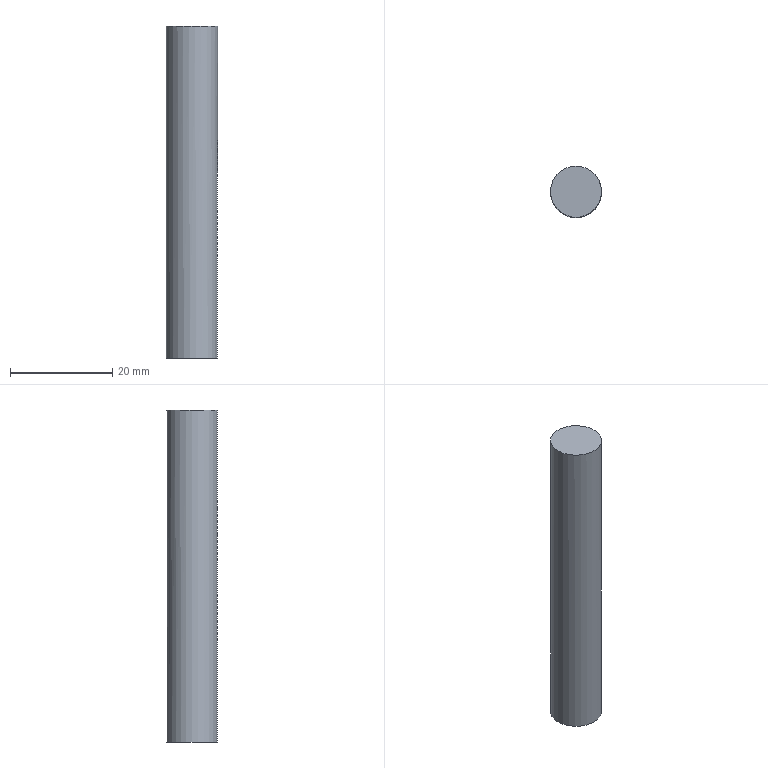Part | NX | features solid 2 | 1 solid | 3 faces | box 10 x 10 x 65 mm | volume 5105 mm3 | plane 2 | cylinder 1 | commonest cylinder face diameters 10 x1
STEP:
#1=CARTESIAN_POINT('',(22.408,15.,85.5));
#2=VERTEX_POINT('',#1);
#3=CARTESIAN_POINT('',(27.408,15.,85.5));
#4=DIRECTION('',(0.,0.,-1.));
#5=DIRECTION('',(-1.,0.,0.));
#6=AXIS2_PLACEMENT_3D('',#3,#4,#5);
#7=CIRCLE('',#6,5.);
#8=EDGE_CURVE('',#2,#2,#7,.T.);
#9=ORIENTED_EDGE('',*,*,#8,.T.);
#10=EDGE_LOOP('',(#9));
#11=FACE_BOUND('',#10,.T.);
#12=CARTESIAN_POINT('',(27.408,20.,20.5));
#13=VERTEX_POINT('',#12);
#14=CARTESIAN_POINT('',(27.408,15.,20.5));
#15=DIRECTION('',(0.,0.,-1.));
#16=DIRECTION('',(0.,1.,0.));
#17=AXIS2_PLACEMENT_3D('',#14,#15,#16);
#18=CIRCLE('',#17,5.);
#19=EDGE_CURVE('',#13,#13,#18,.T.);
#20=ORIENTED_EDGE('',*,*,#19,.F.);
#21=EDGE_LOOP('',(#20));
#22=FACE_BOUND('',#21,.T.);
#23=CARTESIAN_POINT('',(27.408,15.,82.5));
#24=DIRECTION('',(0.,0.,-1.));
#25=DIRECTION('',(-1.,0.,0.));
#26=AXIS2_PLACEMENT_3D('',#23,#24,#25);
#27=CYLINDRICAL_SURFACE('',#26,5.);
#28=ADVANCED_FACE('',(#11,#22),#27,.T.);
#29=ORIENTED_EDGE('',*,*,#8,.F.);
#30=EDGE_LOOP('',(#29));
#31=FACE_BOUND('',#30,.T.);
#32=CARTESIAN_POINT('',(27.408,15.,85.5));
#33=DIRECTION('',(0.,0.,-1.));
#34=DIRECTION('',(-1.,0.,0.));
#35=AXIS2_PLACEMENT_3D('',#32,#33,#34);
#36=PLANE('',#35);
#37=ADVANCED_FACE('',(#31),#36,.F.);
#38=ORIENTED_EDGE('',*,*,#19,.T.);
#39=EDGE_LOOP('',(#38));
#40=FACE_BOUND('',#39,.T.);
#41=CARTESIAN_POINT('',(27.408,15.,20.5));
#42=DIRECTION('',(0.,0.,-1.));
#43=DIRECTION('',(-1.,0.,0.));
#44=AXIS2_PLACEMENT_3D('',#41,#42,#43);
#45=PLANE('',#44);
#46=ADVANCED_FACE('',(#40),#45,.T.);
#47=CLOSED_SHELL('',(#28,#37,#46));
#48=MANIFOLD_SOLID_BREP('',#47);
#49=(LENGTH_UNIT()NAMED_UNIT(*)SI_UNIT(.MILLI.,.METRE.));
#50=UNCERTAINTY_MEASURE_WITH_UNIT(LENGTH_MEASURE(0.00001),#49,'','');
#51=(NAMED_UNIT(*)PLANE_ANGLE_UNIT()SI_UNIT($,.RADIAN.));
#52=(NAMED_UNIT(*)SI_UNIT($,.STERADIAN.)SOLID_ANGLE_UNIT());
#53=(GEOMETRIC_REPRESENTATION_CONTEXT(3)GLOBAL_UNCERTAINTY_ASSIGNED_CONTEXT((#50))GLOBAL_UNIT_ASSIGNED_CONTEXT((#49,#51,#52))REPRESENTATION_CONTEXT('',''));
#54=ADVANCED_BREP_SHAPE_REPRESENTATION('',(#48),#53);